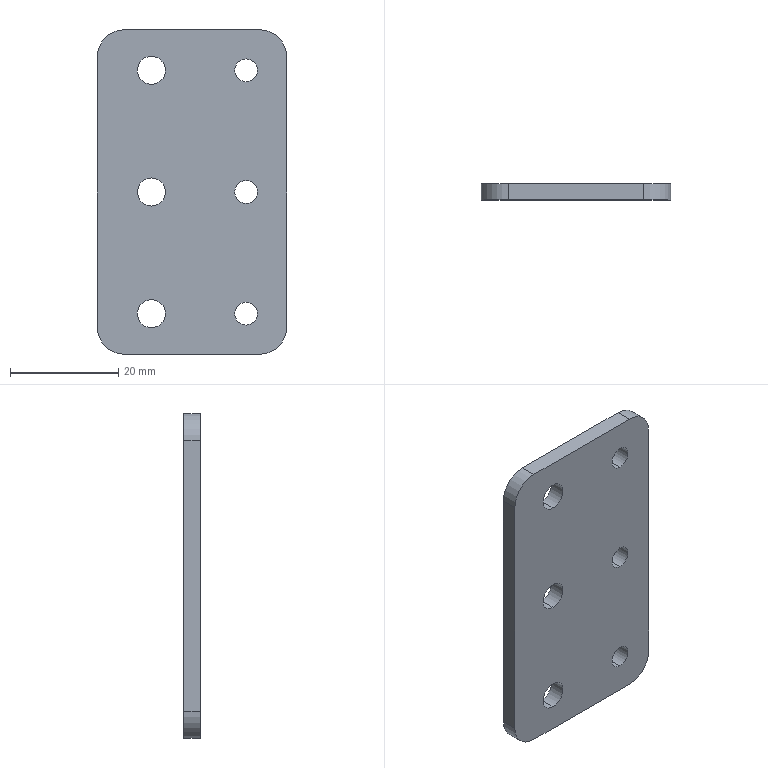Part | SolidWorks | features BaseBody 1 | 1 solid | 22 faces | box 35 x 3 x 60 mm | volume 5920 mm3 | cylinder 16 | plane 6 | commonest cylinder face diameters 4.2 x6 5.2 x6 10 x4
STEP:
#1=CARTESIAN_POINT('',(-7.5,3.,19.9));
#2=VERTEX_POINT('',#1);
#3=CARTESIAN_POINT('',(-7.5,3.,25.1));
#4=VERTEX_POINT('',#3);
#5=CARTESIAN_POINT('',(-7.5,3.,22.5));
#6=DIRECTION('',(0.,1.,0.));
#7=DIRECTION('',(0.,0.,-1.));
#8=AXIS2_PLACEMENT_3D('',#5,#6,#7);
#9=CIRCLE('',#8,2.6);
#10=EDGE_CURVE('',#2,#4,#9,.T.);
#11=ORIENTED_EDGE('',*,*,#10,.T.);
#12=CARTESIAN_POINT('',(-7.5,0.,25.1));
#13=VERTEX_POINT('',#12);
#14=CARTESIAN_POINT('',(-7.5,3.,25.1));
#15=DIRECTION('',(0.,-1.,0.));
#16=VECTOR('',#15,1000.);
#17=LINE('',#14,#16);
#18=EDGE_CURVE('',#4,#13,#17,.T.);
#19=ORIENTED_EDGE('',*,*,#18,.T.);
#20=CARTESIAN_POINT('',(-7.5,0.,19.9));
#21=VERTEX_POINT('',#20);
#22=CARTESIAN_POINT('',(-7.5,0.,22.5));
#23=DIRECTION('',(0.,1.,0.));
#24=DIRECTION('',(0.,0.,-1.));
#25=AXIS2_PLACEMENT_3D('',#22,#23,#24);
#26=CIRCLE('',#25,2.6);
#27=EDGE_CURVE('',#21,#13,#26,.T.);
#28=ORIENTED_EDGE('',*,*,#27,.F.);
#29=CARTESIAN_POINT('',(-7.5,3.,19.9));
#30=DIRECTION('',(0.,-1.,0.));
#31=VECTOR('',#30,1000.);
#32=LINE('',#29,#31);
#33=EDGE_CURVE('',#2,#21,#32,.T.);
#34=ORIENTED_EDGE('',*,*,#33,.F.);
#35=EDGE_LOOP('',(#11,#19,#28,#34));
#36=FACE_OUTER_BOUND('',#35,.T.);
#37=CARTESIAN_POINT('',(-7.5,3.,22.5));
#38=DIRECTION('',(0.,-1.,0.));
#39=DIRECTION('',(0.,0.,-1.));
#40=AXIS2_PLACEMENT_3D('',#37,#38,#39);
#41=CYLINDRICAL_SURFACE('',#40,2.6);
#42=ADVANCED_FACE('',(#36),#41,.F.);
#43=CARTESIAN_POINT('',(-7.5,3.,-2.6));
#44=VERTEX_POINT('',#43);
#45=CARTESIAN_POINT('',(-7.5,3.,2.6));
#46=VERTEX_POINT('',#45);
#47=CARTESIAN_POINT('',(-7.5,3.,0.));
#48=DIRECTION('',(0.,1.,0.));
#49=DIRECTION('',(0.,0.,-1.));
#50=AXIS2_PLACEMENT_3D('',#47,#48,#49);
#51=CIRCLE('',#50,2.6);
#52=EDGE_CURVE('',#44,#46,#51,.T.);
#53=ORIENTED_EDGE('',*,*,#52,.T.);
#54=CARTESIAN_POINT('',(-7.5,0.,2.6));
#55=VERTEX_POINT('',#54);
#56=CARTESIAN_POINT('',(-7.5,3.,2.6));
#57=DIRECTION('',(0.,-1.,0.));
#58=VECTOR('',#57,1000.);
#59=LINE('',#56,#58);
#60=EDGE_CURVE('',#46,#55,#59,.T.);
#61=ORIENTED_EDGE('',*,*,#60,.T.);
#62=CARTESIAN_POINT('',(-7.5,0.,-2.6));
#63=VERTEX_POINT('',#62);
#64=CARTESIAN_POINT('',(-7.5,0.,0.));
#65=DIRECTION('',(0.,1.,0.));
#66=DIRECTION('',(0.,0.,-1.));
#67=AXIS2_PLACEMENT_3D('',#64,#65,#66);
#68=CIRCLE('',#67,2.6);
#69=EDGE_CURVE('',#63,#55,#68,.T.);
#70=ORIENTED_EDGE('',*,*,#69,.F.);
#71=CARTESIAN_POINT('',(-7.5,3.,-2.6));
#72=DIRECTION('',(0.,-1.,0.));
#73=VECTOR('',#72,1000.);
#74=LINE('',#71,#73);
#75=EDGE_CURVE('',#44,#63,#74,.T.);
#76=ORIENTED_EDGE('',*,*,#75,.F.);
#77=EDGE_LOOP('',(#53,#61,#70,#76));
#78=FACE_OUTER_BOUND('',#77,.T.);
#79=CARTESIAN_POINT('',(-7.5,3.,0.));
#80=DIRECTION('',(0.,-1.,0.));
#81=DIRECTION('',(0.,0.,-1.));
#82=AXIS2_PLACEMENT_3D('',#79,#80,#81);
#83=CYLINDRICAL_SURFACE('',#82,2.6);
#84=ADVANCED_FACE('',(#78),#83,.F.);
#85=CARTESIAN_POINT('',(-7.5,3.,-25.1));
#86=VERTEX_POINT('',#85);
#87=CARTESIAN_POINT('',(-7.5,3.,-19.9));
#88=VERTEX_POINT('',#87);
#89=CARTESIAN_POINT('',(-7.5,3.,-22.5));
#90=DIRECTION('',(0.,1.,0.));
#91=DIRECTION('',(0.,0.,-1.));
#92=AXIS2_PLACEMENT_3D('',#89,#90,#91);
#93=CIRCLE('',#92,2.6);
#94=EDGE_CURVE('',#86,#88,#93,.T.);
#95=ORIENTED_EDGE('',*,*,#94,.T.);
#96=CARTESIAN_POINT('',(-7.5,0.,-19.9));
#97=VERTEX_POINT('',#96);
#98=CARTESIAN_POINT('',(-7.5,3.,-19.9));
#99=DIRECTION('',(0.,-1.,0.));
#100=VECTOR('',#99,1000.);
#101=LINE('',#98,#100);
#102=EDGE_CURVE('',#88,#97,#101,.T.);
#103=ORIENTED_EDGE('',*,*,#102,.T.);
#104=CARTESIAN_POINT('',(-7.5,0.,-25.1));
#105=VERTEX_POINT('',#104);
#106=CARTESIAN_POINT('',(-7.5,0.,-22.5));
#107=DIRECTION('',(0.,1.,0.));
#108=DIRECTION('',(0.,0.,-1.));
#109=AXIS2_PLACEMENT_3D('',#106,#107,#108);
#110=CIRCLE('',#109,2.6);
#111=EDGE_CURVE('',#105,#97,#110,.T.);
#112=ORIENTED_EDGE('',*,*,#111,.F.);
#113=CARTESIAN_POINT('',(-7.5,3.,-25.1));
#114=DIRECTION('',(0.,-1.,0.));
#115=VECTOR('',#114,1000.);
#116=LINE('',#113,#115);
#117=EDGE_CURVE('',#86,#105,#116,.T.);
#118=ORIENTED_EDGE('',*,*,#117,.F.);
#119=EDGE_LOOP('',(#95,#103,#112,#118));
#120=FACE_OUTER_BOUND('',#119,.T.);
#121=CARTESIAN_POINT('',(-7.5,3.,-22.5));
#122=DIRECTION('',(0.,-1.,0.));
#123=DIRECTION('',(0.,0.,-1.));
#124=AXIS2_PLACEMENT_3D('',#121,#122,#123);
#125=CYLINDRICAL_SURFACE('',#124,2.6);
#126=ADVANCED_FACE('',(#120),#125,.F.);
#127=CARTESIAN_POINT('',(10.,0.,-2.1));
#128=VERTEX_POINT('',#127);
#129=CARTESIAN_POINT('',(10.,0.,2.1));
#130=VERTEX_POINT('',#129);
#131=CARTESIAN_POINT('',(10.,0.,0.));
#132=DIRECTION('',(0.,1.,0.));
#133=DIRECTION('',(0.,0.,1.));
#134=AXIS2_PLACEMENT_3D('',#131,#132,#133);
#135=CIRCLE('',#134,2.1);
#136=EDGE_CURVE('',#128,#130,#135,.T.);
#137=ORIENTED_EDGE('',*,*,#136,.F.);
#138=CARTESIAN_POINT('',(10.,3.,-2.1));
#139=VERTEX_POINT('',#138);
#140=CARTESIAN_POINT('',(10.,0.,-2.1));
#141=DIRECTION('',(0.,1.,0.));
#142=VECTOR('',#141,1000.);
#143=LINE('',#140,#142);
#144=EDGE_CURVE('',#128,#139,#143,.T.);
#145=ORIENTED_EDGE('',*,*,#144,.T.);
#146=CARTESIAN_POINT('',(10.,3.,2.1));
#147=VERTEX_POINT('',#146);
#148=CARTESIAN_POINT('',(10.,3.,0.));
#149=DIRECTION('',(0.,1.,0.));
#150=DIRECTION('',(0.,0.,1.));
#151=AXIS2_PLACEMENT_3D('',#148,#149,#150);
#152=CIRCLE('',#151,2.1);
#153=EDGE_CURVE('',#139,#147,#152,.T.);
#154=ORIENTED_EDGE('',*,*,#153,.T.);
#155=CARTESIAN_POINT('',(10.,0.,2.1));
#156=DIRECTION('',(0.,1.,0.));
#157=VECTOR('',#156,1000.);
#158=LINE('',#155,#157);
#159=EDGE_CURVE('',#130,#147,#158,.T.);
#160=ORIENTED_EDGE('',*,*,#159,.F.);
#161=EDGE_LOOP('',(#137,#145,#154,#160));
#162=FACE_OUTER_BOUND('',#161,.T.);
#163=CARTESIAN_POINT('',(10.,0.,0.));
#164=DIRECTION('',(0.,1.,0.));
#165=DIRECTION('',(0.,0.,1.));
#166=AXIS2_PLACEMENT_3D('',#163,#164,#165);
#167=CYLINDRICAL_SURFACE('',#166,2.1);
#168=ADVANCED_FACE('',(#162),#167,.F.);
#169=CARTESIAN_POINT('',(10.,0.,-24.6));
#170=VERTEX_POINT('',#169);
#171=CARTESIAN_POINT('',(10.,0.,-20.4));
#172=VERTEX_POINT('',#171);
#173=CARTESIAN_POINT('',(10.,0.,-22.5));
#174=DIRECTION('',(0.,1.,0.));
#175=DIRECTION('',(0.,0.,1.));
#176=AXIS2_PLACEMENT_3D('',#173,#174,#175);
#177=CIRCLE('',#176,2.1);
#178=EDGE_CURVE('',#170,#172,#177,.T.);
#179=ORIENTED_EDGE('',*,*,#178,.F.);
#180=CARTESIAN_POINT('',(10.,3.,-24.6));
#181=VERTEX_POINT('',#180);
#182=CARTESIAN_POINT('',(10.,0.,-24.6));
#183=DIRECTION('',(0.,1.,0.));
#184=VECTOR('',#183,1000.);
#185=LINE('',#182,#184);
#186=EDGE_CURVE('',#170,#181,#185,.T.);
#187=ORIENTED_EDGE('',*,*,#186,.T.);
#188=CARTESIAN_POINT('',(10.,3.,-20.4));
#189=VERTEX_POINT('',#188);
#190=CARTESIAN_POINT('',(10.,3.,-22.5));
#191=DIRECTION('',(0.,1.,0.));
#192=DIRECTION('',(0.,0.,1.));
#193=AXIS2_PLACEMENT_3D('',#190,#191,#192);
#194=CIRCLE('',#193,2.1);
#195=EDGE_CURVE('',#181,#189,#194,.T.);
#196=ORIENTED_EDGE('',*,*,#195,.T.);
#197=CARTESIAN_POINT('',(10.,0.,-20.4));
#198=DIRECTION('',(0.,1.,0.));
#199=VECTOR('',#198,1000.);
#200=LINE('',#197,#199);
#201=EDGE_CURVE('',#172,#189,#200,.T.);
#202=ORIENTED_EDGE('',*,*,#201,.F.);
#203=EDGE_LOOP('',(#179,#187,#196,#202));
#204=FACE_OUTER_BOUND('',#203,.T.);
#205=CARTESIAN_POINT('',(10.,0.,-22.5));
#206=DIRECTION('',(0.,1.,0.));
#207=DIRECTION('',(0.,0.,1.));
#208=AXIS2_PLACEMENT_3D('',#205,#206,#207);
#209=CYLINDRICAL_SURFACE('',#208,2.1);
#210=ADVANCED_FACE('',(#204),#209,.F.);
#211=CARTESIAN_POINT('',(10.,0.,20.4));
#212=VERTEX_POINT('',#211);
#213=CARTESIAN_POINT('',(10.,0.,24.6));
#214=VERTEX_POINT('',#213);
#215=CARTESIAN_POINT('',(10.,0.,22.5));
#216=DIRECTION('',(0.,1.,0.));
#217=DIRECTION('',(0.,0.,1.));
#218=AXIS2_PLACEMENT_3D('',#215,#216,#217);
#219=CIRCLE('',#218,2.1);
#220=EDGE_CURVE('',#212,#214,#219,.T.);
#221=ORIENTED_EDGE('',*,*,#220,.F.);
#222=CARTESIAN_POINT('',(10.,3.,20.4));
#223=VERTEX_POINT('',#222);
#224=CARTESIAN_POINT('',(10.,0.,20.4));
#225=DIRECTION('',(0.,1.,0.));
#226=VECTOR('',#225,1000.);
#227=LINE('',#224,#226);
#228=EDGE_CURVE('',#212,#223,#227,.T.);
#229=ORIENTED_EDGE('',*,*,#228,.T.);
#230=CARTESIAN_POINT('',(10.,3.,24.6));
#231=VERTEX_POINT('',#230);
#232=CARTESIAN_POINT('',(10.,3.,22.5));
#233=DIRECTION('',(0.,1.,0.));
#234=DIRECTION('',(0.,0.,1.));
#235=AXIS2_PLACEMENT_3D('',#232,#233,#234);
#236=CIRCLE('',#235,2.1);
#237=EDGE_CURVE('',#223,#231,#236,.T.);
#238=ORIENTED_EDGE('',*,*,#237,.T.);
#239=CARTESIAN_POINT('',(10.,0.,24.6));
#240=DIRECTION('',(0.,1.,0.));
#241=VECTOR('',#240,1000.);
#242=LINE('',#239,#241);
#243=EDGE_CURVE('',#214,#231,#242,.T.);
#244=ORIENTED_EDGE('',*,*,#243,.F.);
#245=EDGE_LOOP('',(#221,#229,#238,#244));
#246=FACE_OUTER_BOUND('',#245,.T.);
#247=CARTESIAN_POINT('',(10.,0.,22.5));
#248=DIRECTION('',(0.,1.,0.));
#249=DIRECTION('',(0.,0.,1.));
#250=AXIS2_PLACEMENT_3D('',#247,#248,#249);
#251=CYLINDRICAL_SURFACE('',#250,2.1);
#252=ADVANCED_FACE('',(#246),#251,.F.);
#253=ORIENTED_EDGE('',*,*,#10,.F.);
#254=CARTESIAN_POINT('',(-7.5,3.,22.5));
#255=DIRECTION('',(0.,1.,0.));
#256=DIRECTION('',(0.,0.,-1.));
#257=AXIS2_PLACEMENT_3D('',#254,#255,#256);
#258=CIRCLE('',#257,2.6);
#259=EDGE_CURVE('',#4,#2,#258,.T.);
#260=ORIENTED_EDGE('',*,*,#259,.F.);
#261=EDGE_LOOP('',(#253,#260));
#262=FACE_BOUND('',#261,.T.);
#263=ORIENTED_EDGE('',*,*,#52,.F.);
#264=CARTESIAN_POINT('',(-7.5,3.,0.));
#265=DIRECTION('',(0.,1.,0.));
#266=DIRECTION('',(0.,0.,-1.));
#267=AXIS2_PLACEMENT_3D('',#264,#265,#266);
#268=CIRCLE('',#267,2.6);
#269=EDGE_CURVE('',#46,#44,#268,.T.);
#270=ORIENTED_EDGE('',*,*,#269,.F.);
#271=EDGE_LOOP('',(#263,#270));
#272=FACE_BOUND('',#271,.T.);
#273=ORIENTED_EDGE('',*,*,#94,.F.);
#274=CARTESIAN_POINT('',(-7.5,3.,-22.5));
#275=DIRECTION('',(0.,1.,0.));
#276=DIRECTION('',(0.,0.,-1.));
#277=AXIS2_PLACEMENT_3D('',#274,#275,#276);
#278=CIRCLE('',#277,2.6);
#279=EDGE_CURVE('',#88,#86,#278,.T.);
#280=ORIENTED_EDGE('',*,*,#279,.F.);
#281=EDGE_LOOP('',(#273,#280));
#282=FACE_BOUND('',#281,.T.);
#283=CARTESIAN_POINT('',(17.5,3.,25.));
#284=VERTEX_POINT('',#283);
#285=CARTESIAN_POINT('',(12.5,3.,30.));
#286=VERTEX_POINT('',#285);
#287=CARTESIAN_POINT('',(12.5,3.,25.));
#288=DIRECTION('',(0.,-1.,0.));
#289=DIRECTION('',(0.,0.,-1.));
#290=AXIS2_PLACEMENT_3D('',#287,#288,#289);
#291=CIRCLE('',#290,5.);
#292=EDGE_CURVE('',#284,#286,#291,.T.);
#293=ORIENTED_EDGE('',*,*,#292,.F.);
#294=CARTESIAN_POINT('',(17.5,3.,-25.));
#295=VERTEX_POINT('',#294);
#296=CARTESIAN_POINT('',(17.5,3.,0.));
#297=DIRECTION('',(0.,0.,1.));
#298=VECTOR('',#297,1000.);
#299=LINE('',#296,#298);
#300=EDGE_CURVE('',#295,#284,#299,.T.);
#301=ORIENTED_EDGE('',*,*,#300,.F.);
#302=CARTESIAN_POINT('',(12.5,3.,-30.));
#303=VERTEX_POINT('',#302);
#304=CARTESIAN_POINT('',(12.5,3.,-25.));
#305=DIRECTION('',(0.,-1.,0.));
#306=DIRECTION('',(0.,0.,-1.));
#307=AXIS2_PLACEMENT_3D('',#304,#305,#306);
#308=CIRCLE('',#307,5.);
#309=EDGE_CURVE('',#303,#295,#308,.T.);
#310=ORIENTED_EDGE('',*,*,#309,.F.);
#311=CARTESIAN_POINT('',(-12.5,3.,-30.));
#312=VERTEX_POINT('',#311);
#313=CARTESIAN_POINT('',(0.,3.,-30.));
#314=DIRECTION('',(1.,0.,0.));
#315=VECTOR('',#314,1000.);
#316=LINE('',#313,#315);
#317=EDGE_CURVE('',#312,#303,#316,.T.);
#318=ORIENTED_EDGE('',*,*,#317,.F.);
#319=CARTESIAN_POINT('',(-17.5,3.,-25.));
#320=VERTEX_POINT('',#319);
#321=CARTESIAN_POINT('',(-12.5,3.,-25.));
#322=DIRECTION('',(0.,-1.,0.));
#323=DIRECTION('',(0.,0.,-1.));
#324=AXIS2_PLACEMENT_3D('',#321,#322,#323);
#325=CIRCLE('',#324,5.);
#326=EDGE_CURVE('',#320,#312,#325,.T.);
#327=ORIENTED_EDGE('',*,*,#326,.F.);
#328=CARTESIAN_POINT('',(-17.5,3.,25.));
#329=VERTEX_POINT('',#328);
#330=CARTESIAN_POINT('',(-17.5,3.,0.));
#331=DIRECTION('',(0.,0.,-1.));
#332=VECTOR('',#331,1000.);
#333=LINE('',#330,#332);
#334=EDGE_CURVE('',#329,#320,#333,.T.);
#335=ORIENTED_EDGE('',*,*,#334,.F.);
#336=CARTESIAN_POINT('',(-12.5,3.,30.));
#337=VERTEX_POINT('',#336);
#338=CARTESIAN_POINT('',(-12.5,3.,25.));
#339=DIRECTION('',(0.,-1.,0.));
#340=DIRECTION('',(0.,0.,-1.));
#341=AXIS2_PLACEMENT_3D('',#338,#339,#340);
#342=CIRCLE('',#341,5.);
#343=EDGE_CURVE('',#337,#329,#342,.T.);
#344=ORIENTED_EDGE('',*,*,#343,.F.);
#345=CARTESIAN_POINT('',(0.,3.,30.));
#346=DIRECTION('',(-1.,0.,0.));
#347=VECTOR('',#346,1000.);
#348=LINE('',#345,#347);
#349=EDGE_CURVE('',#286,#337,#348,.T.);
#350=ORIENTED_EDGE('',*,*,#349,.F.);
#351=EDGE_LOOP('',(#293,#301,#310,#318,#327,#335,#344,#350));
#352=FACE_OUTER_BOUND('',#351,.T.);
#353=CARTESIAN_POINT('',(10.,3.,0.));
#354=DIRECTION('',(0.,1.,0.));
#355=DIRECTION('',(0.,0.,1.));
#356=AXIS2_PLACEMENT_3D('',#353,#354,#355);
#357=CIRCLE('',#356,2.1);
#358=EDGE_CURVE('',#147,#139,#357,.T.);
#359=ORIENTED_EDGE('',*,*,#358,.F.);
#360=ORIENTED_EDGE('',*,*,#153,.F.);
#361=EDGE_LOOP('',(#359,#360));
#362=FACE_BOUND('',#361,.T.);
#363=CARTESIAN_POINT('',(10.,3.,-22.5));
#364=DIRECTION('',(0.,1.,0.));
#365=DIRECTION('',(0.,0.,1.));
#366=AXIS2_PLACEMENT_3D('',#363,#364,#365);
#367=CIRCLE('',#366,2.1);
#368=EDGE_CURVE('',#189,#181,#367,.T.);
#369=ORIENTED_EDGE('',*,*,#368,.F.);
#370=ORIENTED_EDGE('',*,*,#195,.F.);
#371=EDGE_LOOP('',(#369,#370));
#372=FACE_BOUND('',#371,.T.);
#373=CARTESIAN_POINT('',(10.,3.,22.5));
#374=DIRECTION('',(0.,1.,0.));
#375=DIRECTION('',(0.,0.,1.));
#376=AXIS2_PLACEMENT_3D('',#373,#374,#375);
#377=CIRCLE('',#376,2.1);
#378=EDGE_CURVE('',#231,#223,#377,.T.);
#379=ORIENTED_EDGE('',*,*,#378,.F.);
#380=ORIENTED_EDGE('',*,*,#237,.F.);
#381=EDGE_LOOP('',(#379,#380));
#382=FACE_BOUND('',#381,.T.);
#383=CARTESIAN_POINT('',(0.,3.,0.));
#384=DIRECTION('',(0.,-1.,0.));
#385=DIRECTION('',(0.,0.,-1.));
#386=AXIS2_PLACEMENT_3D('',#383,#384,#385);
#387=PLANE('',#386);
#388=ADVANCED_FACE('',(#262,#272,#282,#352,#362,#372,#382),#387,.F.);
#389=ORIENTED_EDGE('',*,*,#18,.F.);
#390=ORIENTED_EDGE('',*,*,#259,.T.);
#391=ORIENTED_EDGE('',*,*,#33,.T.);
#392=CARTESIAN_POINT('',(-7.5,0.,22.5));
#393=DIRECTION('',(0.,1.,0.));
#394=DIRECTION('',(0.,0.,-1.));
#395=AXIS2_PLACEMENT_3D('',#392,#393,#394);
#396=CIRCLE('',#395,2.6);
#397=EDGE_CURVE('',#13,#21,#396,.T.);
#398=ORIENTED_EDGE('',*,*,#397,.F.);
#399=EDGE_LOOP('',(#389,#390,#391,#398));
#400=FACE_OUTER_BOUND('',#399,.T.);
#401=CARTESIAN_POINT('',(-7.5,3.,22.5));
#402=DIRECTION('',(0.,-1.,0.));
#403=DIRECTION('',(0.,0.,-1.));
#404=AXIS2_PLACEMENT_3D('',#401,#402,#403);
#405=CYLINDRICAL_SURFACE('',#404,2.6);
#406=ADVANCED_FACE('',(#400),#405,.F.);
#407=ORIENTED_EDGE('',*,*,#60,.F.);
#408=ORIENTED_EDGE('',*,*,#269,.T.);
#409=ORIENTED_EDGE('',*,*,#75,.T.);
#410=CARTESIAN_POINT('',(-7.5,0.,0.));
#411=DIRECTION('',(0.,1.,0.));
#412=DIRECTION('',(0.,0.,-1.));
#413=AXIS2_PLACEMENT_3D('',#410,#411,#412);
#414=CIRCLE('',#413,2.6);
#415=EDGE_CURVE('',#55,#63,#414,.T.);
#416=ORIENTED_EDGE('',*,*,#415,.F.);
#417=EDGE_LOOP('',(#407,#408,#409,#416));
#418=FACE_OUTER_BOUND('',#417,.T.);
#419=CARTESIAN_POINT('',(-7.5,3.,0.));
#420=DIRECTION('',(0.,-1.,0.));
#421=DIRECTION('',(0.,0.,-1.));
#422=AXIS2_PLACEMENT_3D('',#419,#420,#421);
#423=CYLINDRICAL_SURFACE('',#422,2.6);
#424=ADVANCED_FACE('',(#418),#423,.F.);
#425=ORIENTED_EDGE('',*,*,#102,.F.);
#426=ORIENTED_EDGE('',*,*,#279,.T.);
#427=ORIENTED_EDGE('',*,*,#117,.T.);
#428=CARTESIAN_POINT('',(-7.5,0.,-22.5));
#429=DIRECTION('',(0.,1.,0.));
#430=DIRECTION('',(0.,0.,-1.));
#431=AXIS2_PLACEMENT_3D('',#428,#429,#430);
#432=CIRCLE('',#431,2.6);
#433=EDGE_CURVE('',#97,#105,#432,.T.);
#434=ORIENTED_EDGE('',*,*,#433,.F.);
#435=EDGE_LOOP('',(#425,#426,#427,#434));
#436=FACE_OUTER_BOUND('',#435,.T.);
#437=CARTESIAN_POINT('',(-7.5,3.,-22.5));
#438=DIRECTION('',(0.,-1.,0.));
#439=DIRECTION('',(0.,0.,-1.));
#440=AXIS2_PLACEMENT_3D('',#437,#438,#439);
#441=CYLINDRICAL_SURFACE('',#440,2.6);
#442=ADVANCED_FACE('',(#436),#441,.F.);
#443=CARTESIAN_POINT('',(12.5,0.,30.));
#444=VERTEX_POINT('',#443);
#445=CARTESIAN_POINT('',(12.5,3.,30.));
#446=DIRECTION('',(0.,-1.,0.));
#447=VECTOR('',#446,1000.);
#448=LINE('',#445,#447);
#449=EDGE_CURVE('',#286,#444,#448,.T.);
#450=ORIENTED_EDGE('',*,*,#449,.F.);
#451=ORIENTED_EDGE('',*,*,#349,.T.);
#452=CARTESIAN_POINT('',(-12.5,0.,30.));
#453=VERTEX_POINT('',#452);
#454=CARTESIAN_POINT('',(-12.5,3.,30.));
#455=DIRECTION('',(0.,1.,0.));
#456=VECTOR('',#455,1000.);
#457=LINE('',#454,#456);
#458=EDGE_CURVE('',#453,#337,#457,.T.);
#459=ORIENTED_EDGE('',*,*,#458,.F.);
#460=CARTESIAN_POINT('',(-17.5,0.,30.));
#461=DIRECTION('',(-1.,0.,0.));
#462=VECTOR('',#461,1000.);
#463=LINE('',#460,#462);
#464=EDGE_CURVE('',#444,#453,#463,.T.);
#465=ORIENTED_EDGE('',*,*,#464,.F.);
#466=EDGE_LOOP('',(#450,#451,#459,#465));
#467=FACE_OUTER_BOUND('',#466,.T.);
#468=CARTESIAN_POINT('',(-17.5,3.,30.));
#469=DIRECTION('',(0.,0.,-1.));
#470=DIRECTION('',(-1.,0.,0.));
#471=AXIS2_PLACEMENT_3D('',#468,#469,#470);
#472=PLANE('',#471);
#473=ADVANCED_FACE('',(#467),#472,.F.);
#474=CARTESIAN_POINT('',(17.5,0.,25.));
#475=VERTEX_POINT('',#474);
#476=CARTESIAN_POINT('',(12.5,0.,25.));
#477=DIRECTION('',(0.,1.,0.));
#478=DIRECTION('',(0.,0.,-1.));
#479=AXIS2_PLACEMENT_3D('',#476,#477,#478);
#480=CIRCLE('',#479,5.);
#481=EDGE_CURVE('',#444,#475,#480,.T.);
#482=ORIENTED_EDGE('',*,*,#481,.T.);
#483=CARTESIAN_POINT('',(17.5,3.,25.));
#484=DIRECTION('',(0.,1.,0.));
#485=VECTOR('',#484,1000.);
#486=LINE('',#483,#485);
#487=EDGE_CURVE('',#475,#284,#486,.T.);
#488=ORIENTED_EDGE('',*,*,#487,.T.);
#489=ORIENTED_EDGE('',*,*,#292,.T.);
#490=ORIENTED_EDGE('',*,*,#449,.T.);
#491=EDGE_LOOP('',(#482,#488,#489,#490));
#492=FACE_OUTER_BOUND('',#491,.T.);
#493=CARTESIAN_POINT('',(12.5,3.,25.));
#494=DIRECTION('',(0.,-1.,0.));
#495=DIRECTION('',(0.,0.,-1.));
#496=AXIS2_PLACEMENT_3D('',#493,#494,#495);
#497=CYLINDRICAL_SURFACE('',#496,5.);
#498=ADVANCED_FACE('',(#492),#497,.T.);
#499=ORIENTED_EDGE('',*,*,#487,.F.);
#500=CARTESIAN_POINT('',(17.5,0.,-25.));
#501=VERTEX_POINT('',#500);
#502=CARTESIAN_POINT('',(17.5,0.,30.));
#503=DIRECTION('',(0.,0.,1.));
#504=VECTOR('',#503,1000.);
#505=LINE('',#502,#504);
#506=EDGE_CURVE('',#501,#475,#505,.T.);
#507=ORIENTED_EDGE('',*,*,#506,.F.);
#508=CARTESIAN_POINT('',(17.5,3.,-25.));
#509=DIRECTION('',(0.,-1.,0.));
#510=VECTOR('',#509,1000.);
#511=LINE('',#508,#510);
#512=EDGE_CURVE('',#295,#501,#511,.T.);
#513=ORIENTED_EDGE('',*,*,#512,.F.);
#514=ORIENTED_EDGE('',*,*,#300,.T.);
#515=EDGE_LOOP('',(#499,#507,#513,#514));
#516=FACE_OUTER_BOUND('',#515,.T.);
#517=CARTESIAN_POINT('',(17.5,3.,30.));
#518=DIRECTION('',(-1.,0.,0.));
#519=DIRECTION('',(0.,0.,1.));
#520=AXIS2_PLACEMENT_3D('',#517,#518,#519);
#521=PLANE('',#520);
#522=ADVANCED_FACE('',(#516),#521,.F.);
#523=CARTESIAN_POINT('',(12.5,0.,-30.));
#524=VERTEX_POINT('',#523);
#525=CARTESIAN_POINT('',(12.5,0.,-25.));
#526=DIRECTION('',(0.,1.,0.));
#527=DIRECTION('',(0.,0.,-1.));
#528=AXIS2_PLACEMENT_3D('',#525,#526,#527);
#529=CIRCLE('',#528,5.);
#530=EDGE_CURVE('',#501,#524,#529,.T.);
#531=ORIENTED_EDGE('',*,*,#530,.T.);
#532=CARTESIAN_POINT('',(12.5,3.,-30.));
#533=DIRECTION('',(0.,1.,0.));
#534=VECTOR('',#533,1000.);
#535=LINE('',#532,#534);
#536=EDGE_CURVE('',#524,#303,#535,.T.);
#537=ORIENTED_EDGE('',*,*,#536,.T.);
#538=ORIENTED_EDGE('',*,*,#309,.T.);
#539=ORIENTED_EDGE('',*,*,#512,.T.);
#540=EDGE_LOOP('',(#531,#537,#538,#539));
#541=FACE_OUTER_BOUND('',#540,.T.);
#542=CARTESIAN_POINT('',(12.5,3.,-25.));
#543=DIRECTION('',(0.,-1.,0.));
#544=DIRECTION('',(0.,0.,-1.));
#545=AXIS2_PLACEMENT_3D('',#542,#543,#544);
#546=CYLINDRICAL_SURFACE('',#545,5.);
#547=ADVANCED_FACE('',(#541),#546,.T.);
#548=CARTESIAN_POINT('',(-12.5,0.,-30.));
#549=VERTEX_POINT('',#548);
#550=CARTESIAN_POINT('',(-12.5,3.,-30.));
#551=DIRECTION('',(0.,-1.,0.));
#552=VECTOR('',#551,1000.);
#553=LINE('',#550,#552);
#554=EDGE_CURVE('',#312,#549,#553,.T.);
#555=ORIENTED_EDGE('',*,*,#554,.F.);
#556=ORIENTED_EDGE('',*,*,#317,.T.);
#557=ORIENTED_EDGE('',*,*,#536,.F.);
#558=CARTESIAN_POINT('',(-17.5,0.,-30.));
#559=DIRECTION('',(1.,0.,0.));
#560=VECTOR('',#559,1000.);
#561=LINE('',#558,#560);
#562=EDGE_CURVE('',#549,#524,#561,.T.);
#563=ORIENTED_EDGE('',*,*,#562,.F.);
#564=EDGE_LOOP('',(#555,#556,#557,#563));
#565=FACE_OUTER_BOUND('',#564,.T.);
#566=CARTESIAN_POINT('',(-17.5,3.,-30.));
#567=DIRECTION('',(0.,0.,1.));
#568=DIRECTION('',(1.,0.,0.));
#569=AXIS2_PLACEMENT_3D('',#566,#567,#568);
#570=PLANE('',#569);
#571=ADVANCED_FACE('',(#565),#570,.F.);
#572=CARTESIAN_POINT('',(-17.5,0.,-25.));
#573=VERTEX_POINT('',#572);
#574=CARTESIAN_POINT('',(-12.5,0.,-25.));
#575=DIRECTION('',(0.,1.,0.));
#576=DIRECTION('',(0.,0.,-1.));
#577=AXIS2_PLACEMENT_3D('',#574,#575,#576);
#578=CIRCLE('',#577,5.);
#579=EDGE_CURVE('',#549,#573,#578,.T.);
#580=ORIENTED_EDGE('',*,*,#579,.T.);
#581=CARTESIAN_POINT('',(-17.5,3.,-25.));
#582=DIRECTION('',(0.,1.,0.));
#583=VECTOR('',#582,1000.);
#584=LINE('',#581,#583);
#585=EDGE_CURVE('',#573,#320,#584,.T.);
#586=ORIENTED_EDGE('',*,*,#585,.T.);
#587=ORIENTED_EDGE('',*,*,#326,.T.);
#588=ORIENTED_EDGE('',*,*,#554,.T.);
#589=EDGE_LOOP('',(#580,#586,#587,#588));
#590=FACE_OUTER_BOUND('',#589,.T.);
#591=CARTESIAN_POINT('',(-12.5,3.,-25.));
#592=DIRECTION('',(0.,-1.,0.));
#593=DIRECTION('',(0.,0.,-1.));
#594=AXIS2_PLACEMENT_3D('',#591,#592,#593);
#595=CYLINDRICAL_SURFACE('',#594,5.);
#596=ADVANCED_FACE('',(#590),#595,.T.);
#597=ORIENTED_EDGE('',*,*,#585,.F.);
#598=CARTESIAN_POINT('',(-17.5,0.,25.));
#599=VERTEX_POINT('',#598);
#600=CARTESIAN_POINT('',(-17.5,0.,30.));
#601=DIRECTION('',(0.,0.,-1.));
#602=VECTOR('',#601,1000.);
#603=LINE('',#600,#602);
#604=EDGE_CURVE('',#599,#573,#603,.T.);
#605=ORIENTED_EDGE('',*,*,#604,.F.);
#606=CARTESIAN_POINT('',(-17.5,3.,25.));
#607=DIRECTION('',(0.,-1.,0.));
#608=VECTOR('',#607,1000.);
#609=LINE('',#606,#608);
#610=EDGE_CURVE('',#329,#599,#609,.T.);
#611=ORIENTED_EDGE('',*,*,#610,.F.);
#612=ORIENTED_EDGE('',*,*,#334,.T.);
#613=EDGE_LOOP('',(#597,#605,#611,#612));
#614=FACE_OUTER_BOUND('',#613,.T.);
#615=CARTESIAN_POINT('',(-17.5,3.,30.));
#616=DIRECTION('',(1.,0.,0.));
#617=DIRECTION('',(0.,0.,-1.));
#618=AXIS2_PLACEMENT_3D('',#615,#616,#617);
#619=PLANE('',#618);
#620=ADVANCED_FACE('',(#614),#619,.F.);
#621=CARTESIAN_POINT('',(-12.5,0.,25.));
#622=DIRECTION('',(0.,1.,0.));
#623=DIRECTION('',(0.,0.,-1.));
#624=AXIS2_PLACEMENT_3D('',#621,#622,#623);
#625=CIRCLE('',#624,5.);
#626=EDGE_CURVE('',#599,#453,#625,.T.);
#627=ORIENTED_EDGE('',*,*,#626,.T.);
#628=ORIENTED_EDGE('',*,*,#458,.T.);
#629=ORIENTED_EDGE('',*,*,#343,.T.);
#630=ORIENTED_EDGE('',*,*,#610,.T.);
#631=EDGE_LOOP('',(#627,#628,#629,#630));
#632=FACE_OUTER_BOUND('',#631,.T.);
#633=CARTESIAN_POINT('',(-12.5,3.,25.));
#634=DIRECTION('',(0.,-1.,0.));
#635=DIRECTION('',(0.,0.,-1.));
#636=AXIS2_PLACEMENT_3D('',#633,#634,#635);
#637=CYLINDRICAL_SURFACE('',#636,5.);
#638=ADVANCED_FACE('',(#632),#637,.T.);
#639=ORIENTED_EDGE('',*,*,#144,.F.);
#640=CARTESIAN_POINT('',(10.,0.,0.));
#641=DIRECTION('',(0.,1.,0.));
#642=DIRECTION('',(0.,0.,1.));
#643=AXIS2_PLACEMENT_3D('',#640,#641,#642);
#644=CIRCLE('',#643,2.1);
#645=EDGE_CURVE('',#130,#128,#644,.T.);
#646=ORIENTED_EDGE('',*,*,#645,.F.);
#647=ORIENTED_EDGE('',*,*,#159,.T.);
#648=ORIENTED_EDGE('',*,*,#358,.T.);
#649=EDGE_LOOP('',(#639,#646,#647,#648));
#650=FACE_OUTER_BOUND('',#649,.T.);
#651=CARTESIAN_POINT('',(10.,0.,0.));
#652=DIRECTION('',(0.,1.,0.));
#653=DIRECTION('',(0.,0.,1.));
#654=AXIS2_PLACEMENT_3D('',#651,#652,#653);
#655=CYLINDRICAL_SURFACE('',#654,2.1);
#656=ADVANCED_FACE('',(#650),#655,.F.);
#657=ORIENTED_EDGE('',*,*,#186,.F.);
#658=CARTESIAN_POINT('',(10.,0.,-22.5));
#659=DIRECTION('',(0.,1.,0.));
#660=DIRECTION('',(0.,0.,1.));
#661=AXIS2_PLACEMENT_3D('',#658,#659,#660);
#662=CIRCLE('',#661,2.1);
#663=EDGE_CURVE('',#172,#170,#662,.T.);
#664=ORIENTED_EDGE('',*,*,#663,.F.);
#665=ORIENTED_EDGE('',*,*,#201,.T.);
#666=ORIENTED_EDGE('',*,*,#368,.T.);
#667=EDGE_LOOP('',(#657,#664,#665,#666));
#668=FACE_OUTER_BOUND('',#667,.T.);
#669=CARTESIAN_POINT('',(10.,0.,-22.5));
#670=DIRECTION('',(0.,1.,0.));
#671=DIRECTION('',(0.,0.,1.));
#672=AXIS2_PLACEMENT_3D('',#669,#670,#671);
#673=CYLINDRICAL_SURFACE('',#672,2.1);
#674=ADVANCED_FACE('',(#668),#673,.F.);
#675=ORIENTED_EDGE('',*,*,#228,.F.);
#676=CARTESIAN_POINT('',(10.,0.,22.5));
#677=DIRECTION('',(0.,1.,0.));
#678=DIRECTION('',(0.,0.,1.));
#679=AXIS2_PLACEMENT_3D('',#676,#677,#678);
#680=CIRCLE('',#679,2.1);
#681=EDGE_CURVE('',#214,#212,#680,.T.);
#682=ORIENTED_EDGE('',*,*,#681,.F.);
#683=ORIENTED_EDGE('',*,*,#243,.T.);
#684=ORIENTED_EDGE('',*,*,#378,.T.);
#685=EDGE_LOOP('',(#675,#682,#683,#684));
#686=FACE_OUTER_BOUND('',#685,.T.);
#687=CARTESIAN_POINT('',(10.,0.,22.5));
#688=DIRECTION('',(0.,1.,0.));
#689=DIRECTION('',(0.,0.,1.));
#690=AXIS2_PLACEMENT_3D('',#687,#688,#689);
#691=CYLINDRICAL_SURFACE('',#690,2.1);
#692=ADVANCED_FACE('',(#686),#691,.F.);
#693=ORIENTED_EDGE('',*,*,#27,.T.);
#694=ORIENTED_EDGE('',*,*,#397,.T.);
#695=EDGE_LOOP('',(#693,#694));
#696=FACE_BOUND('',#695,.T.);
#697=ORIENTED_EDGE('',*,*,#111,.T.);
#698=ORIENTED_EDGE('',*,*,#433,.T.);
#699=EDGE_LOOP('',(#697,#698));
#700=FACE_BOUND('',#699,.T.);
#701=ORIENTED_EDGE('',*,*,#562,.T.);
#702=ORIENTED_EDGE('',*,*,#530,.F.);
#703=ORIENTED_EDGE('',*,*,#506,.T.);
#704=ORIENTED_EDGE('',*,*,#481,.F.);
#705=ORIENTED_EDGE('',*,*,#464,.T.);
#706=ORIENTED_EDGE('',*,*,#626,.F.);
#707=ORIENTED_EDGE('',*,*,#604,.T.);
#708=ORIENTED_EDGE('',*,*,#579,.F.);
#709=EDGE_LOOP('',(#701,#702,#703,#704,#705,#706,#707,#708));
#710=FACE_OUTER_BOUND('',#709,.T.);
#711=ORIENTED_EDGE('',*,*,#69,.T.);
#712=ORIENTED_EDGE('',*,*,#415,.T.);
#713=EDGE_LOOP('',(#711,#712));
#714=FACE_BOUND('',#713,.T.);
#715=ORIENTED_EDGE('',*,*,#645,.T.);
#716=ORIENTED_EDGE('',*,*,#136,.T.);
#717=EDGE_LOOP('',(#715,#716));
#718=FACE_BOUND('',#717,.T.);
#719=ORIENTED_EDGE('',*,*,#663,.T.);
#720=ORIENTED_EDGE('',*,*,#178,.T.);
#721=EDGE_LOOP('',(#719,#720));
#722=FACE_BOUND('',#721,.T.);
#723=ORIENTED_EDGE('',*,*,#681,.T.);
#724=ORIENTED_EDGE('',*,*,#220,.T.);
#725=EDGE_LOOP('',(#723,#724));
#726=FACE_BOUND('',#725,.T.);
#727=CARTESIAN_POINT('',(0.,0.,0.));
#728=DIRECTION('',(0.,-1.,0.));
#729=DIRECTION('',(0.,0.,-1.));
#730=AXIS2_PLACEMENT_3D('',#727,#728,#729);
#731=PLANE('',#730);
#732=ADVANCED_FACE('',(#696,#700,#710,#714,#718,#722,#726),#731,.T.);
#733=CLOSED_SHELL('',(#42,#84,#126,#168,#210,#252,#388,#406,#424,#442,#473,#498,#522,#547,#571,#596,#620,#638,#656,#674,#692,#732));
#734=MANIFOLD_SOLID_BREP('',#733);
#735=CARTESIAN_POINT('',(0.,0.,0.));
#736=DIRECTION('',(0.,0.,1.));
#737=DIRECTION('',(1.,0.,0.));
#738=AXIS2_PLACEMENT_3D('',#735,#736,#737);
#739=(LENGTH_UNIT()NAMED_UNIT(*)SI_UNIT(.MILLI.,.METRE.));
#740=UNCERTAINTY_MEASURE_WITH_UNIT(LENGTH_MEASURE(0.00001),#739,'','');
#741=(NAMED_UNIT(*)PLANE_ANGLE_UNIT()SI_UNIT($,.RADIAN.));
#742=(NAMED_UNIT(*)SI_UNIT($,.STERADIAN.)SOLID_ANGLE_UNIT());
#743=(GEOMETRIC_REPRESENTATION_CONTEXT(3)GLOBAL_UNCERTAINTY_ASSIGNED_CONTEXT((#740))GLOBAL_UNIT_ASSIGNED_CONTEXT((#739,#741,#742))REPRESENTATION_CONTEXT('',''));
#744=ADVANCED_BREP_SHAPE_REPRESENTATION('',(#734,#738),#743);